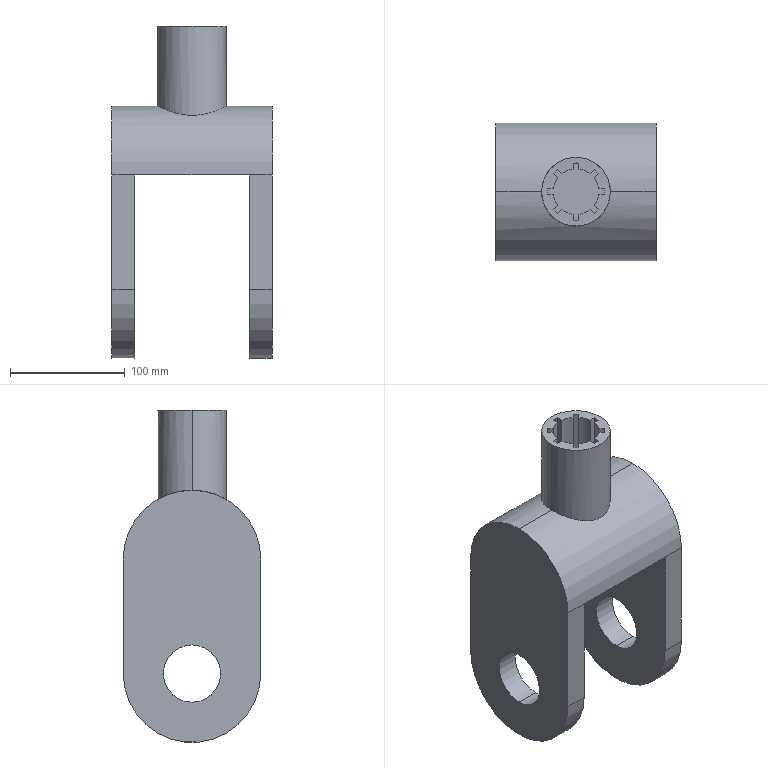Part | SolidWorks | 1 solid | 54 faces | box 140 x 120 x 290 mm | volume 1506174 mm3 | cylinder 27 | plane 27 | commonest cylinder face diameters 50 x13 40 x8 120 x4 60 x2